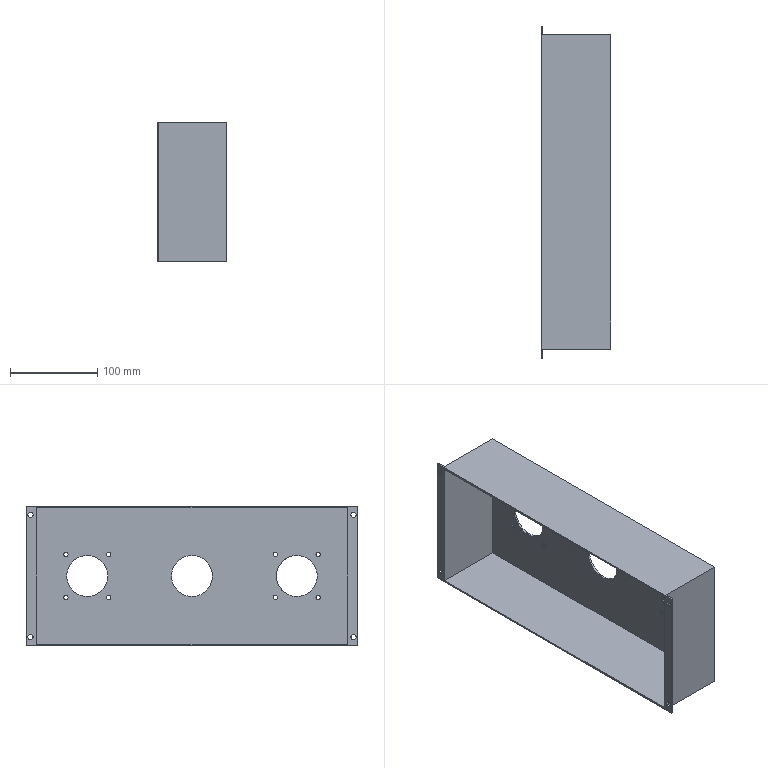Part | STEP file | Positioning_id2214_x_t | 1 solid | 45 faces | box 80 x 380 x 160 mm | volume 271642 mm3 | cylinder 30 | plane 15 | commonest cylinder face diameters 5 x16 6 x8 47 x6